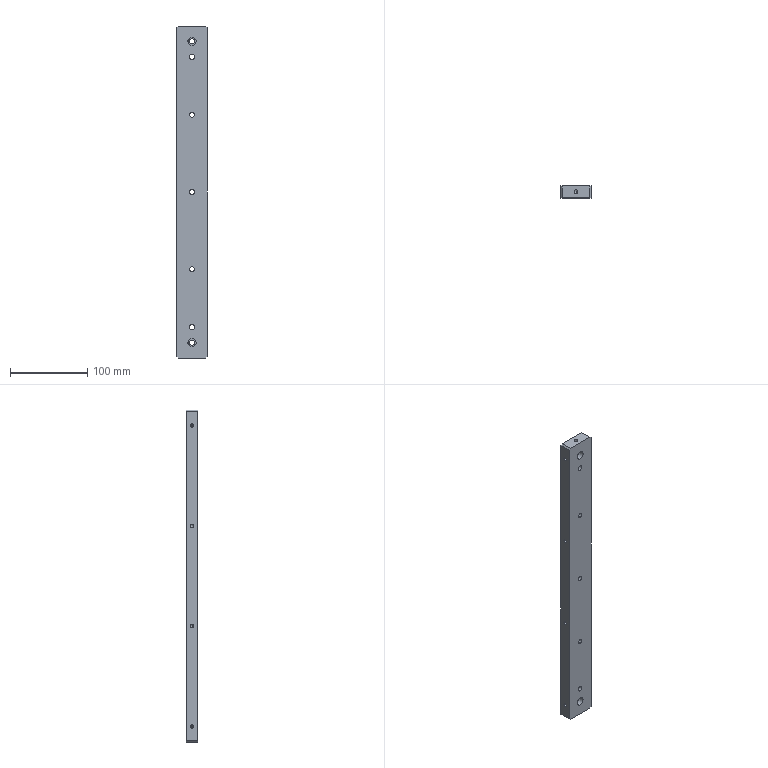Part | SolidWorks | features HoleWzd 6, Chamfer 2, ICE 2, Extrusion 1, Fillet 1 | 1 solid | 69 faces | box 40 x 15 x 430 mm | volume 250428 mm3 | cylinder 40 | plane 17 | cone 12 | commonest cylinder face diameters 6.6 x10 11 x10 4.2 x8 5 x4 6 x4 13 x4